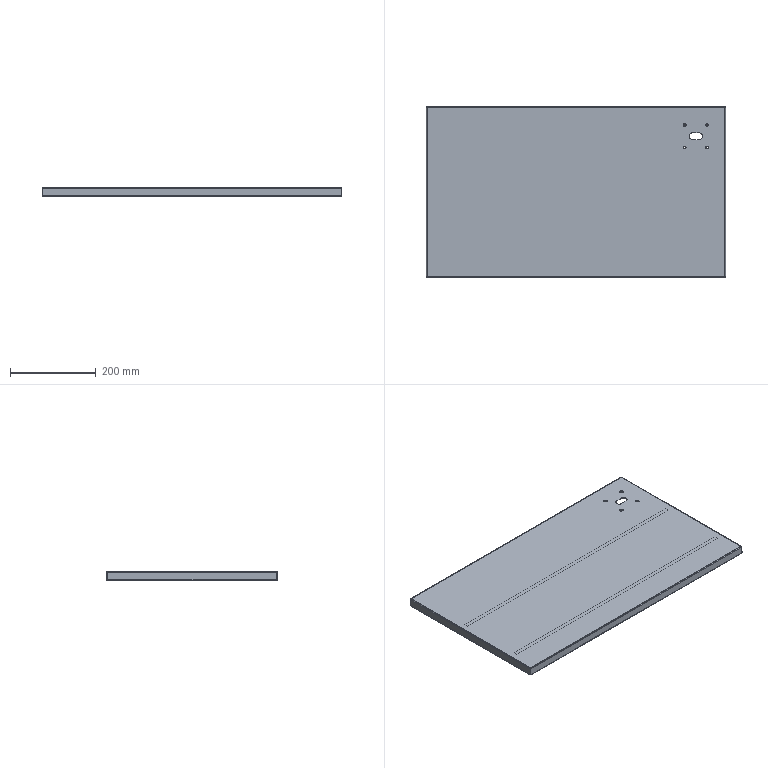Part | STEP file | FBDS-BJ-007 | 2 solids | 293 faces | box 698 x 398 x 20 mm | volume 721973 mm3 | cylinder 147 | plane 130 | spline 16 | commonest cylinder face diameters 4 x20 5.4 x20 7.87 x20 0.4 x12 3.3 x12 3.4 x12